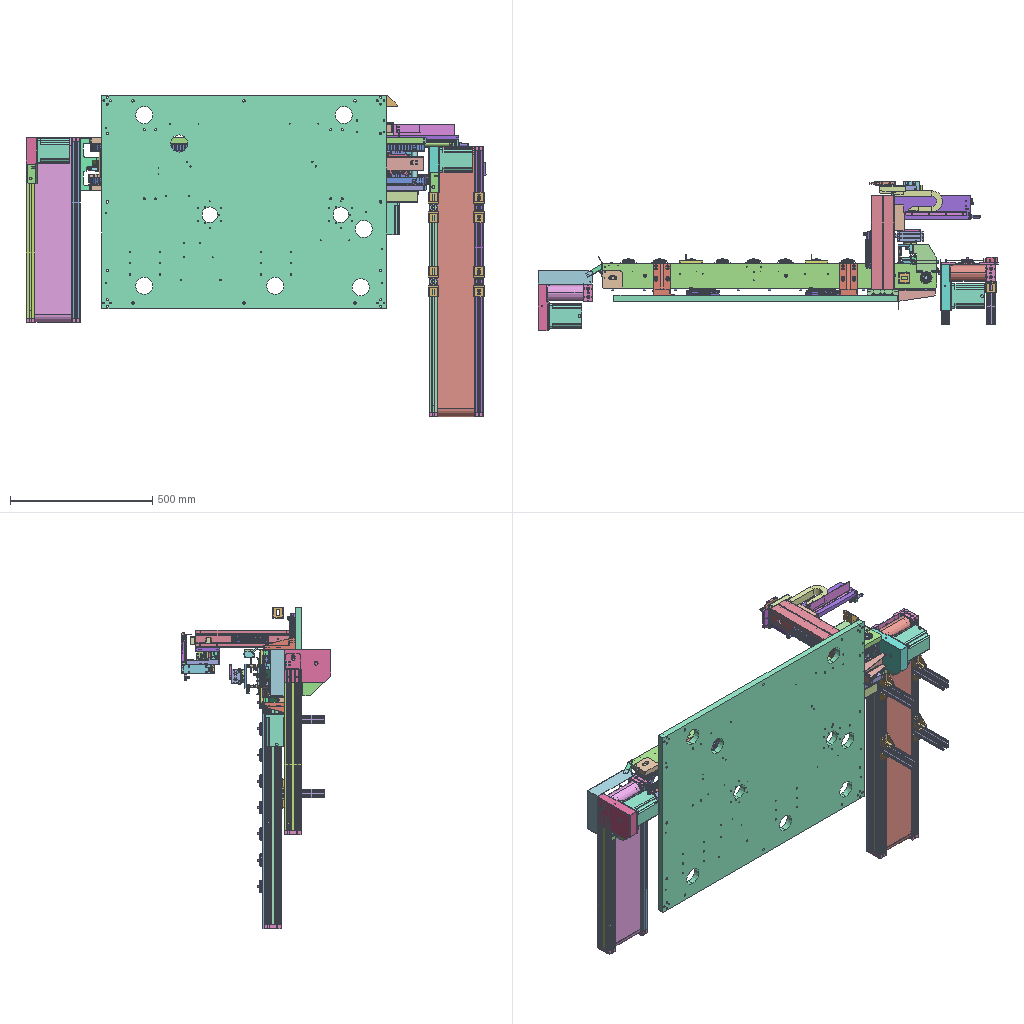Assembly | STEP file | 114 different items | 249 placed | box 1615 x 525 x 1130 mm
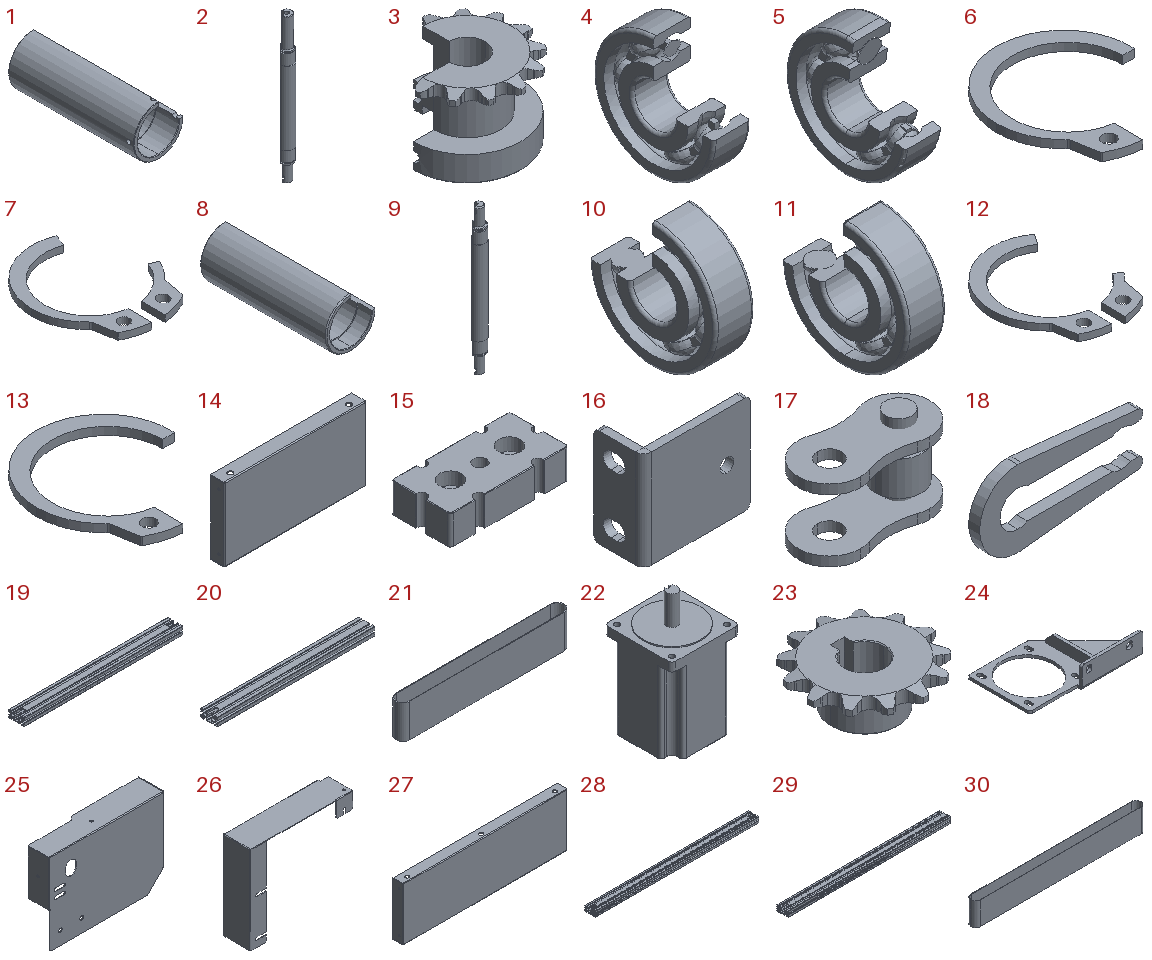Parts list (item | name | quantity | parent item | size | volume):
1 | - | x2 | - | 50 x 126 x 50 mm | 63059 mm3
2 | drive shaft | x2 | - | 16 x 16 x 176 mm | 21338 mm3
3 | driven sprocket | x2 | - | 44.21 x 43.904 x 30.003 mm | 14979 mm3
4 | Bearing 6302 | x2 | - | 13 x 42 x 42 mm | 7777 mm3
5 | Bearing 6302 | x2 | - | 13 x 41.82 x 42 mm | 7834 mm3
6 | Shaft retaining ring type A 15 | x2 | - | 16.8 x 19.352 x 1 mm | 66.829 mm3
7 | Shaft retaining ring type A 15 | x2 | - | 16.068 x 19.352 x 1 mm | 68.849 mm3
8 | - | x2 | - | 50 x 126 x 50 mm | 63952 mm3
9 | driven shaft | x2 | - | 16 x 15.999 x 170 mm | 21183 mm3
10 | Bearing 6302 | x2 | - | 13 x 42 x 42 mm | 7890 mm3
11 | Bearing 6302 | x2 | - | 13 x 41.997 x 42 mm | 7881 mm3
12 | Shaft retaining ring type A 15 | x2 | - | 15.123 x 19.352 x 1 mm | 70.172 mm3
13 | Shaft retaining ring type A 15 | x2 | - | 16.8 x 19.352 x 1 mm | 66.829 mm3
14 | - | x2 | - | 250 x 25 x 130 mm | 74457 mm3
15 | B2200 end cap_zinc alloy | x6 | - | 60 x 30 x 15 mm | 23538 mm3
16 | drive wheel fixing plate | x2 | - | 54.501 x 25.501 x 50 mm | 14216 mm3
17 | Industrial chain 06B-1-160 links | x2 | - | 18.125 x 8.6 x 12.32 mm | 522.22 mm3
18 | Chain link 3 (06B) | x2 | - | 15 x 1 x 7 mm | 49.292 mm3
19 | belt line support ET profile 620 | x1 | - | 620 x 60 x 30 mm | 399085 mm3
20 | belt line support ET profile 565 | x1 | - | 565 x 60 x 30 mm | 364592 mm3
21 | Light green PVC conveyor belt 1346x129x2mm thick_antistatic | x1 | - | 648.5 x 54 x 129 mm | 348910 mm3
22 | Stepper motor 34HS4801D14PJ5 | x3 | in HJ conveyor line assembly | 86 x 89 x 152.5 mm | 773985 mm3
23 | Drive sprocket 06B-13 teeth_bore φ14 | x2 | - | 44.21 x 43.904 x 16.003 mm | 7455 mm3
24 | - | x2 | - | 160 x 100 x 32 mm | 46086 mm3
25 | sprocket guard | x1 | - | 163 x 35.5 x 116 mm | 28902 mm3
26 | - | x1 | - | 190 x 50 x 163 mm | 24970 mm3
27 | belt support plate | x2 | - | 400 x 25 x 130 mm | 113936 mm3
28 | belt line support ET profile 920 | x1 | - | 920 x 60 x 30 mm | 594868 mm3
29 | - | x1 | - | 865 x 60 x 30 mm | 559855 mm3
30 | Light green PVC conveyor belt 1946x129x2mm thick_antistatic | x1 | - | 948.5 x 54 x 129 mm | 503710 mm3
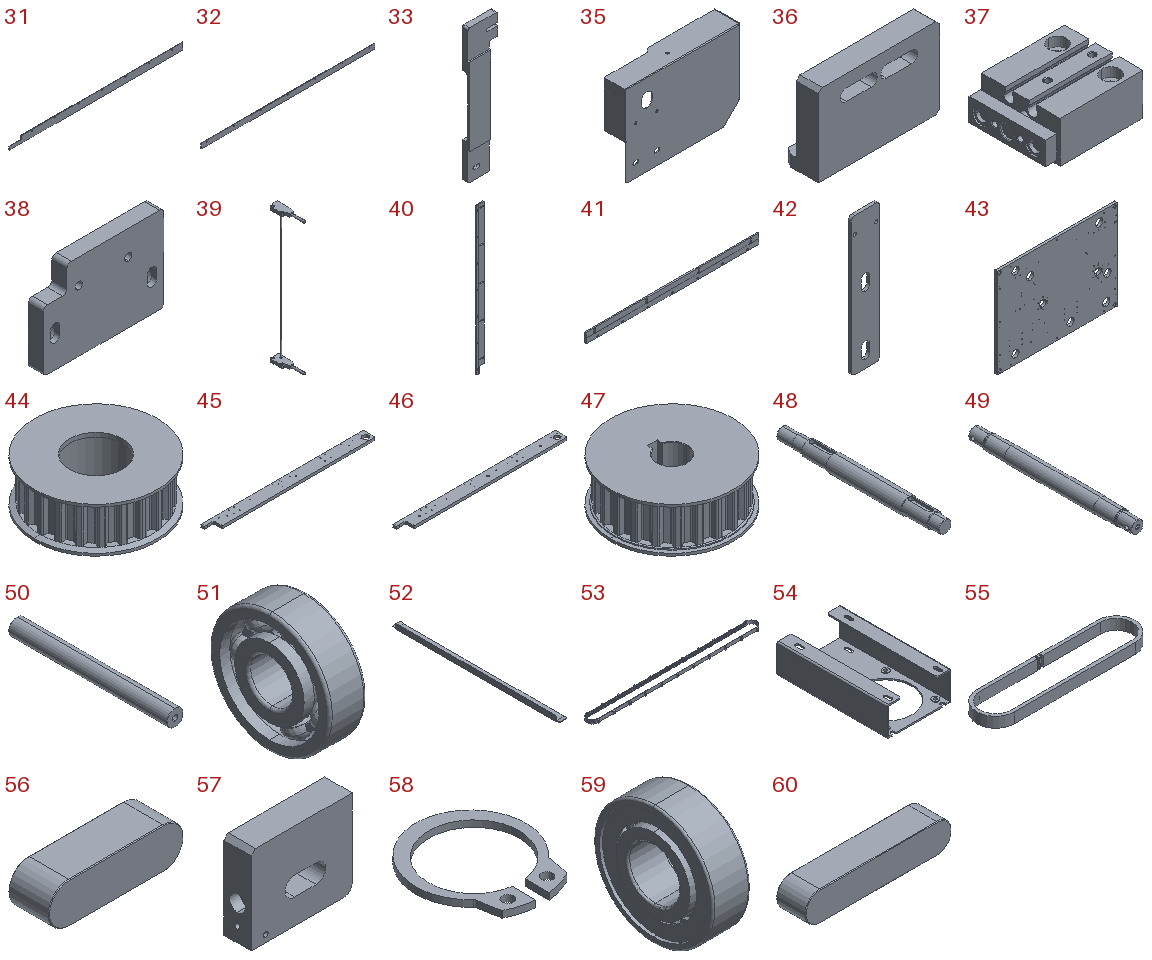31 | BZJ-BZMM-JDKTBDYY Product限位Plate一 | x1 | - | 890 x 2 x 35 mm | 59822 mm3
32 | BZJ-BZMM-JDKTBDYY Product限位Plate二 | x1 | - | 895 x 2 x 26 mm | 46280 mm3
33 | - | x1 | - | 42 x 10 x 190 mm | 34788 mm3
34 | product | x21 | in gripper rotary assembly | - | -
35 | motor fixing plate | x1 | - | 163 x 35.5 x 116 mm | 28996 mm3
36 | secondary positioning block | x1 | - | 33 x 9.454 x 22 mm | 4103 mm3
37 | Three-axis cylinder TCM10x10S | x1 | - | - | -
38 | - | x1 | - | 56 x 7 x 40 mm | 13740 mm3
39 | Through-beam ultra-thin photoelectric switch EX-11A_150 | x1 | - | 10 x 35.5 x 157 mm | 1436 mm3
40 | BZJ-BZMM-JDKTBDYY Product限位Plate四 | x1 | - | 44 x 6 x 895 mm | 219689 mm3
41 | BZJ-BZMM-JDKTBDYY Product限位Plate三 | x1 | - | 830 x 6 x 48 mm | 225450 mm3
42 | through-beam photoelectric fixing plate | x2 | - | 14.5 x 1.5 x 70 mm | 1416 mm3
43 | - | x1 | - | 1000 x 22 x 750 mm | 15887768 mm3
44 | Timing pulley 22-T10-φ35-27 | x2 | in HJ conveyor line assembly | 74 x 74 x 27 mm | 67542 mm3
45 | - | x1 | in HJ conveyor line assembly | 1175 x 85 x 19 mm | 1776717 mm3
46 | - | x1 | in HJ conveyor line assembly | 1175 x 85 x 19 mm | 1780086 mm3
47 | Timing pulley 22-T10-φ18-27 | x2 | in HJ conveyor line assembly | 74 x 74 x 27 mm | 85142 mm3
48 | - | x1 | in HJ conveyor line assembly | 20 x 198 x 20 mm | 50387 mm3
49 | - | x1 | in HJ conveyor line assembly | 16 x 176 x 16 mm | 31579 mm3
50 | - | x3 | in HJ conveyor line assembly | 15 x 147 x 15 mm | 25052 mm3
51 | Bearing 6302 | x2 | in HJ conveyor line assembly | 13 x 42 x 42 mm | 10445 mm3
52 | T10 timing belt support plate | x4 | in HJ conveyor line assembly | 25.5 x 510.959 x 15 mm | 29071 mm3
53 | Timing belt with stop block 2420-T10-21mm wide | x2 | in HJ conveyor line assembly | 1172 x 86.18 x 21.9 mm | 158627 mm3
54 | 86 motor mounting flange | x1 | in HJ conveyor line assembly | 90 x 155 x 41 mm | 53412 mm3
55 | Timing belt 270-3M-8mm wide_28-28 teeth H93 | x1 | in HJ conveyor line assembly | 122.34 x 29.34 x 8 mm | 5374 mm3
56 | Type A key 6x6 20L | x2 | in HJ conveyor line assembly | 20 x 6 x 6 mm | 673.18 mm3
57 | adjustment limit plate | x2 | in HJ conveyor line assembly | 70 x 19 x 60 mm | 70894 mm3
58 | Shaft retaining ring type A 15 | x2 | in HJ conveyor line assembly | 16.8 x 19.352 x 1 mm | 89.212 mm3
59 | Bearing 6202-2Z | x4 | in HJ conveyor line assembly | 11 x 35 x 35 mm | 5288 mm3
60 | Plain key type A 5x5x25 | x1 | in HJ conveyor line assembly | 25 x 5 x 5 mm | 597.62 mm3
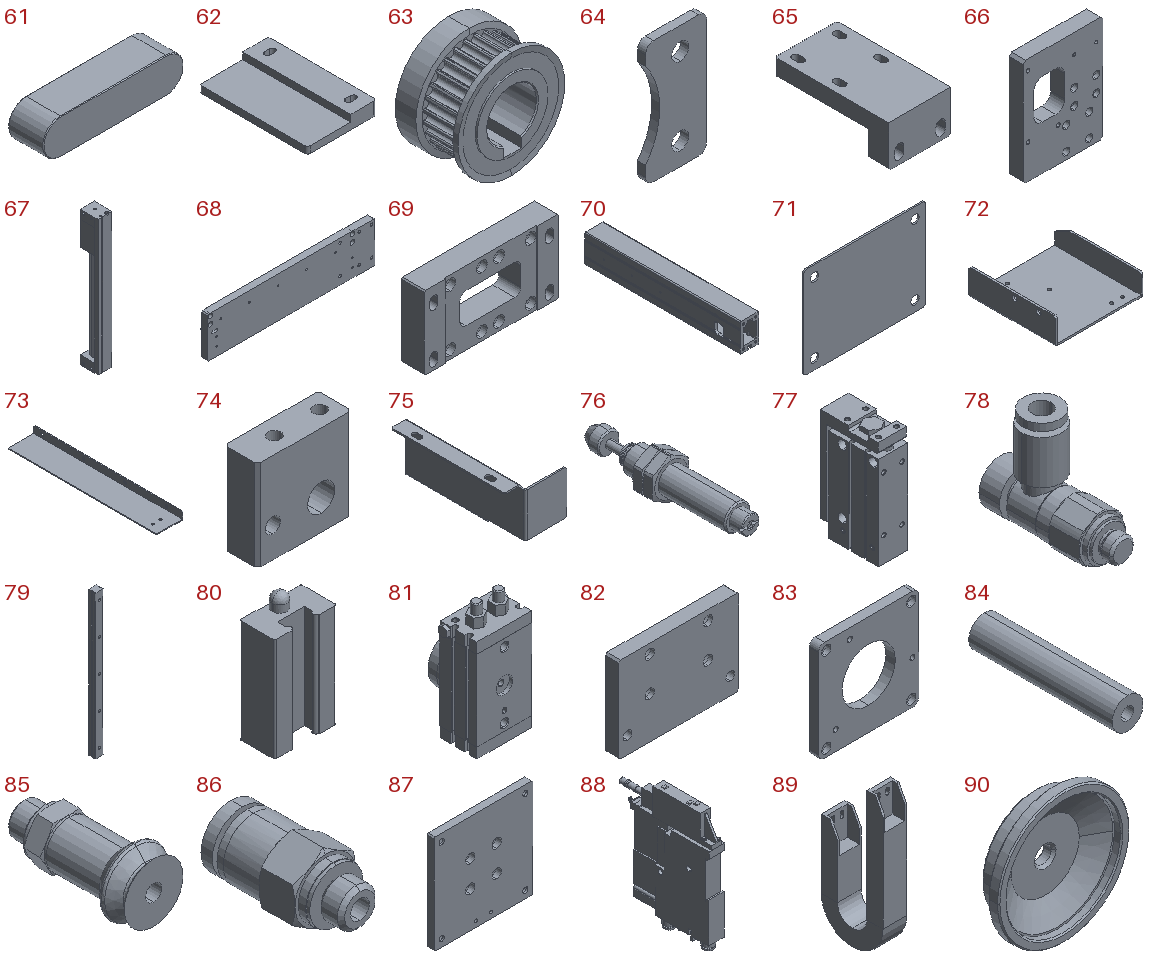61 | Plain key (type B) 5x5x20 | x1 | in HJ conveyor line assembly | 20 x 5 x 5 mm | 472.72 mm3
62 | - | x4 | in HJ conveyor line assembly | 51 x 80 x 10 mm | 27378 mm3
63 | Timing pulley 28-3M-φ14-19-J | x2 | in HJ conveyor line assembly | 30 x 19 x 30 mm | 7318 mm3
64 | - | x2 | in HJ conveyor line assembly | 15 x 2 x 30 mm | 737.571 mm3
65 | - | x4 | - | 60 x 110 x 40 mm | 130636 mm3
66 | slide fixing plate | x1 | in gripper rotary assembly | 90 x 24 x 120 mm | 159761 mm3
67 | Magnetically coupled rodless cylinder CY3R15-200 | x1 | in gripper rotary assembly | 32 x 40 x 294 mm | 185652 mm3
68 | - | x1 | in gripper rotary assembly | 350 x 14 x 85 mm | 395442 mm3
69 | - | x1 | in gripper rotary assembly | 110 x 19 x 60 mm | 87261 mm3
70 | - | x2 | in gripper rotary assembly | 40 x 330 x 60 mm | 402728 mm3
71 | 4060 profile end cover plate | x1 | in gripper rotary assembly | 80 x 1 x 60 mm | 4702 mm3
72 | drag chain fixing plate | x1 | in gripper rotary assembly | 91 x 90 x 27 mm | 24044 mm3
73 | drag chain support plate | x1 | in gripper rotary assembly | 38 x 215 x 11 mm | 12174 mm3
74 | - | x2 | in gripper rotary assembly | 31 x 11 x 30 mm | 8762 mm3
75 | - | x1 | in gripper rotary assembly | 42 x 90 x 36.2 mm | 8185 mm3
76 | Hydraulic shock absorber ACA1007-2 | x2 | in gripper rotary assembly | 14 x 62 x 15.686 mm | 4586 mm3
77 | Pneumatic slide MXH20-50Z_with magnet_no sensor | x1 | in gripper rotary assembly | 32 x 64.5 x 118 mm | 192171 mm3
78 | Speed control valve AS1201F-M5-04A | x4 | in gripper rotary assembly | 9.373 x 25.4 x 22 mm | 1869 mm3
79 | Guide rail SSR15XW1SSC1+270LY | x1 | in 79 | 15 x 12.5 x 270 mm | 46741 mm3
80 | Slider 15_THK_SSR15XW | x1 | in 79 | 34 x 19.5 x 65 mm | 30926 mm3
81 | Swing table MSQB10A | x1 | in gripper rotary assembly | 55.4 x 47 x 109.81 mm | 167301 mm3
82 | swing table fixing plate | x1 | in gripper rotary assembly | 70 x 8 x 50 mm | 25661 mm3
83 | - | x1 | - | 85 x 8 x 85 mm | 43514 mm3
84 | connecting column | x4 | - | 8 x 37 x 8 mm | 1657 mm3
85 | Vacuum suction cup ZPT08BS-A5_longitudinal vacuum outlet type_no buffer_bellows type | x3 | - | 10 x 20 x 10 mm | 691.38 mm3
86 | Quick-change joint KQ2H04-M5A | x3 | - | 8 x 17 x 9.238 mm | 543.469 mm3
87 | - | x1 | - | 85 x 6 x 85 mm | 41251 mm3
88 | Vacuum generator ZK2A10K5KW-06 | x1 | in gripper rotary assembly | - | -
89 | JFLO drag chain 15.20B, bend radius R28 | x1 | in gripper rotary assembly | 28.5 x 74.5 x 172.25 mm | 143432 mm3
90 | - | x1 | in gripper rotary assembly | 55 x 12.5 x 55 mm | 12038 mm3
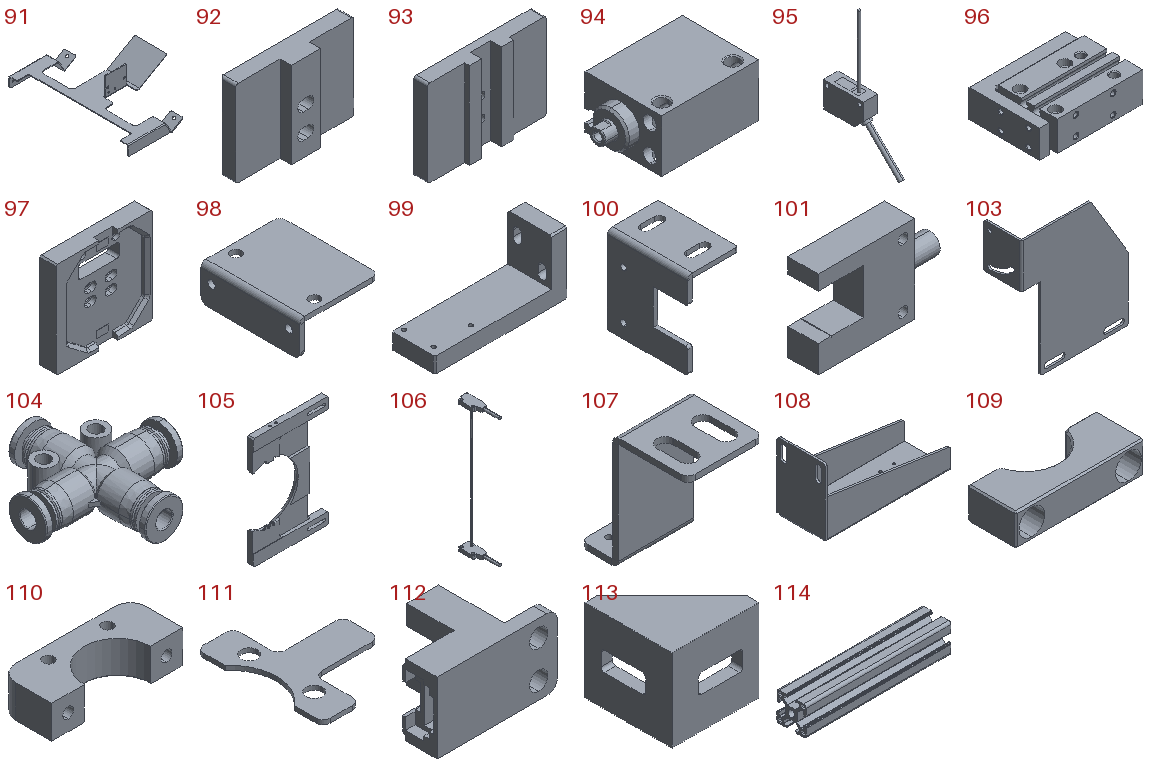91 | unloading flow plate | x1 | - | 128.223 x 185 x 46.263 mm | 15132 mm3
92 | product positioning block | x2 | - | 48 x 12.5 x 35 mm | 13200 mm3
93 | product positioning block B | x30 | - | 48 x 10 x 35 mm | 11917 mm3
94 | Compact free-mount cylinder MU6x6S | x1 | - | 30 x 19 x 13 mm | 4914 mm3
95 | Compact photoelectric sensor CX-441 | x4 | in lift assembly | 11.2 x 58.715 x 100.215 mm | 7246 mm3
96 | Compact pneumatic slide MXH6-15Z | x2 | in lift assembly | 54.5 x 39 x 16 mm | 25990 mm3
97 | lift positioning block | x2 | in lift assembly | 70 x 12 x 70 mm | 41545 mm3
98 | lift photoelectric fixing plate | x2 | in lift assembly | 25.5 x 32 x 11.5 mm | 1639 mm3
99 | cylinder fixing plate 2 | x2 | in lift assembly | 85 x 28 x 40 mm | 31178 mm3
100 | photoelectric mounting plate | x1 | - | 22 x 35 x 38 mm | 3386 mm3
101 | Photoelectric sensor SU15-N | x1 | - | 42 x 11.5 x 29 mm | 7150 mm3
102 | I/O junction box 23N8S1 | x3 | - | - | -
103 | photoelectric fixing plate 2 | x1 | - | 85 x 30 x 100 mm | 11300 mm3
104 | Tube fitting PZ4 | x1 | - | 34 x 34 x 9.5 mm | 2906 mm3
105 | material release guide plate | x1 | - | 125 x 10 x 185 mm | 96002 mm3
106 | Through-beam ultra-thin photoelectric switch EX-11A_120 | x1 | - | 10 x 35.5 x 127 mm | 1412 mm3
107 | - | x2 | - | 20 x 28.5 x 30 mm | 1546 mm3
108 | - | x1 | - | 130 x 50 x 70 mm | 33645 mm3
109 | photoelectric switch fixing block 1 | x1 | - | 40 x 15 x 10 mm | 3490 mm3
110 | photoelectric switch fixing plate 2 | x1 | - | 40 x 16 x 10 mm | 4339 mm3
111 | - | x1 | - | 28 x 35 x 1.2 mm | 521.608 mm3
112 | Photoelectric sensor PM-Y65 | x1 | - | 22.7 x 14.9 x 13.4 mm | 1660 mm3
113 | Die-cast aluminium connector, 40 series, 40mm face, standard type | x9 | - | 38 x 38 x 36 mm | 14409 mm3
114 | MK-8-3030-L-00 profile 3030 standard type 150mm | x4 | - | 150 x 30 x 30 mm | 48990 mm3
Placements (level | parent | child | x y z in mm | rotation matrix by rows):
1 | subassembly 2 | subassembly 3 | -12.345 572.465 974.383 | 1 0 9e-06 0 -1 0 9e-06 0 -1
2 | subassembly 3 | subassembly 4 | -203.579 -184.273 737.895 | 0 1 0 -1 0 0 0 0 1
3 | subassembly 4 | subassembly 5 | -56.737 26.612 373.0 | 1 0 0 0 1 0 0 0 1
3 | subassembly 4 | drive shaft | -56.737 23.612 373.0 | 0 1 0 0 0 -1 -1 0 -0
3 | subassembly 4 | driven sprocket | -56.737 -54.242 373.0 | 0 1 0 0 0 -1 -1 0 0
3 | subassembly 4 | Bearing 6302 | -56.737 -19.888 373.0 | 0 -1 0 1 0 0 0 0 1
3 | subassembly 4 | Bearing 6302 | -56.737 82.112 373.0 | 0 -0.9914 -0.1307 1 0 0 0 -0.1307 0.9914
3 | subassembly 4 | Shaft retaining ring type A 15 | -56.737 -26.888 372.5 | 1 0 0 0 0 1 0 -1 0
3 | subassembly 4 | Shaft retaining ring type A 15 | -56.27 89.112 372.822 | 0.357 0.9341 0 0 0 1 0.9341 -0.357 0
2 | subassembly 3 | subassembly 6 | -196.548 -168.949 1359.395 | 0 -1 0 1 0 0 0 0 1
3 | subassembly 6 | subassembly 7 | 41.413 -19.581 346.0 | 1 0 0 0 1 0 0 0 1
3 | subassembly 6 | driven shaft | 41.413 -19.581 346.0 | 0.01582 0.9999 0 0 0 -1 -0.9999 0.01582 0
3 | subassembly 6 | Bearing 6302 | 41.413 35.919 346.0 | 0 1 0 -1 0 0 0 0 1
3 | subassembly 6 | Bearing 6302 | 41.413 -75.081 346.0 | 0 0.9998 -0.01821 -1 0 0 0 0.01821 0.9998
3 | subassembly 6 | Shaft retaining ring type A 15 | 41.828 -82.081 345.72 | 0.5593 0.829 0 0 0 1 0.829 -0.5593 -0
3 | subassembly 6 | Shaft retaining ring type A 15 | 41.413 42.919 345.5 | 1 0 0 0 0 1 0 -1 0
2 | subassembly 3 | subassembly 8 | -176.967 -151.036 1541.203 | 0 0 1 0 1 0 -1 0 -0
2 | subassembly 3 | subassembly 8 | -176.967 -151.036 1291.203 | 0 0 1 0 1 0 -1 0 -0
2 | subassembly 3 | B2200 end cap_zinc alloy | -96.967 -127.535 1090.896 | 0 1 0 1 0 0 0 0 -1
2 | subassembly 3 | B2200 end cap_zinc alloy | -256.967 -127.535 1725.896 | 0 -1 0 1 0 0 0 0 1
2 | subassembly 3 | B2200 end cap_zinc alloy | -96.967 -127.535 1725.896 | 0 -1 0 1 0 0 0 0 1
2 | subassembly 3 | drive wheel fixing plate | -267.967 -127.535 1098.895 | 0 1 0 0 0 -1 -1 0 -0
2 | subassembly 3 | Industrial chain 06B-1-160 links | -267.89 -45.475 1101.33 | 0 0 -1 0.9905 -0.1375 0 -0.1375 -0.9905 0
2 | subassembly 3 | Chain link 3 (06B) | -262.761 -50.192 1101.984 | 0 -1 0 -0.9905 0 -0.1375 0.1375 0 -0.9905
2 | subassembly 3 | belt line support ET profile 620 | -96.967 -142.536 1408.396 | 0 0 -1 0 -1 0 -1 0 0
2 | subassembly 3 | belt line support ET profile 565 | -256.967 -112.535 1435.896 | 0 0 1 0 1 0 -1 0 -0
2 | subassembly 3 | Light green PVC conveyor belt 1346x129x2mm thick_antistatic | -176.967 -127.535 1408.145 | 0 0 1 0 1 0 -1 0 -0
2 | subassembly 3 | Stepper motor 34HS4801D14PJ5 | -119.967 -46.035 1131.396 | 0 0 -1 1 0 0 0 -1 -0
2 | subassembly 3 | Drive sprocket 06B-13 teeth_bore φ14 | -257.821 -46.035 1131.396 | 0 0 -1 -0.9914 0.1312 0 0.1312 0.9914 -0
2 | subassembly 3 | subassembly 9 | -237.967 -42.535 1131.396 | 0 0 -1 0 1 0 1 0 0
2 | subassembly 3 | sprocket guard | -271.967 -156.536 1084.396 | 0 1 0 1 0 0 0 0 -1
2 | subassembly 3 | subassembly 10 | -271.967 -182.536 1083.396 | 1 0 0 0 -1 0 0 0 -1
1 | subassembly 2 | subassembly 11 | 1122.454 698.033 793.393 | 0 -1 9e-06 -1 0 0 0 -9e-06 -1
2 | subassembly 11 | subassembly 4 | -128.705 -75.924 587.895 | -1 0 0 0 -1 0 0 0 1
3 | subassembly 4 | subassembly 5 | -56.737 26.612 373.0 | 1 0 0 0 1 0 0 0 1
3 | subassembly 4 | drive shaft | -56.737 23.612 373.0 | 0 1 0 0 0 -1 -1 0 -0
3 | subassembly 4 | driven sprocket | -56.737 -54.242 373.0 | 0 1 0 0 0 -1 -1 0 0
3 | subassembly 4 | Bearing 6302 | -56.737 -19.888 373.0 | 0 -1 0 1 0 0 0 0 1
3 | subassembly 4 | Bearing 6302 | -56.737 82.112 373.0 | 0 -0.9914 -0.1307 1 0 0 0 -0.1307 0.9914
3 | subassembly 4 | Shaft retaining ring type A 15 | -56.737 -26.888 372.5 | 1 0 0 0 0 1 0 -1 0
3 | subassembly 4 | Shaft retaining ring type A 15 | -56.27 89.112 372.822 | 0.357 0.9341 0 0 0 1 0.9341 -0.357 0
2 | subassembly 11 | subassembly 6 | -113.38 -82.954 1509.395 | 1 0 0 0 1 0 0 0 1
3 | subassembly 6 | subassembly 7 | 41.413 -19.581 346.0 | 1 0 0 0 1 0 0 0 1
3 | subassembly 6 | driven shaft | 41.413 -19.581 346.0 | 0.01582 0.9999 0 0 0 -1 -0.9999 0.01582 0
3 | subassembly 6 | Bearing 6302 | 41.413 35.919 346.0 | 0 1 0 -1 0 0 0 0 1
3 | subassembly 6 | Bearing 6302 | 41.413 -75.081 346.0 | 0 0.9998 -0.01821 -1 0 0 0 0.01821 0.9998
3 | subassembly 6 | Shaft retaining ring type A 15 | 41.828 -82.081 345.72 | 0.5593 0.829 0 0 0 1 0.829 -0.5593 -0
3 | subassembly 6 | Shaft retaining ring type A 15 | 41.413 42.919 345.5 | 1 0 0 0 0 1 0 -1 0
2 | subassembly 11 | belt support plate | -95.467 -102.535 1603.396 | 0 1 0 0 0 -1 -1 0 0
2 | subassembly 11 | belt support plate | -95.467 -102.535 1203.396 | 0 1 0 0 0 -1 -1 0 0
2 | subassembly 11 | B2200 end cap_zinc alloy | -71.967 -182.536 940.896 | -1 0 0 0 1 0 0 0 -1
2 | subassembly 11 | B2200 end cap_zinc alloy | -71.967 -22.535 1875.896 | 1 0 0 0 1 0 0 0 1
2 | subassembly 11 | B2200 end cap_zinc alloy | -71.967 -182.536 1875.896 | 1 0 0 0 1 0 0 0 1
2 | subassembly 11 | drive wheel fixing plate | -71.967 -11.536 948.895 | 0 0 -1 0 -1 0 -1 0 0
2 | subassembly 11 | Industrial chain 06B-1-160 links | 19.686 -26.615 960.264 | 0.7485 0.6631 0 6e-06 -6e-06 1 0.6631 -0.7485 -9e-06
2 | subassembly 11 | Chain link 3 (06B) | 16.121 -31.744 957.106 | -0.7485 0 0.6631 -6e-06 1 -6e-06 -0.6631 -9e-06 -0.7485
2 | subassembly 11 | belt line support ET profile 920 | -86.967 -182.536 1408.396 | 0 -1 0 0 0 1 -1 0 0
2 | subassembly 11 | subassembly 12 | -56.967 -22.535 1435.896 | 0 1 0 0 0 -1 -1 0 0
2 | subassembly 11 | Light green PVC conveyor belt 1946x129x2mm thick_antistatic | -71.967 -102.535 1408.145 | 0 1 0 0 0 -1 -1 0 0
2 | subassembly 11 | BZJ-BZMM-JDKTBDYY Product限位Plate一 | -100.467 -144.536 1438.396 | 0 -1 0 0 0 -1 1 0 0
2 | subassembly 11 | BZJ-BZMM-JDKTBDYY Product限位Plate二 | -102.467 -55.035 1435.896 | 0 1 0 0 0 1 1 0 0
2 | subassembly 11 | subassembly 13 | -101.967 -102.535 948.396 | 0 -1 0 0 0 -1 1 0 -0
2 | subassembly 11 | product | -91.767 -183.843 927.176 | -1 0 0 0 1 -0.001005 0 -0.001005 -1
2 | subassembly 11 | motor fixing plate | -100.967 -7.535 934.396 | 1 0 0 0 -1 0 0 0 -1
2 | subassembly 11 | subassembly 9 | 13.033 -41.535 981.396 | 0 1 0 0 0 1 1 0 0
2 | subassembly 11 | Stepper motor 34HS4801D14PJ5 | 9.533 -159.536 981.396 | 1 0 0 0 0 1 0 -1 -0
2 | subassembly 11 | Drive sprocket 06B-13 teeth_bore φ14 | 9.533 -21.682 981.396 | -0.9892 0.1467 0 0 0 1 0.1467 0.9892 0
2 | subassembly 11 | secondary positioning block | -110.467 -159.536 1007.596 | 0 0 -1 0 1 0 1 0 -0
2 | subassembly 11 | Three-axis cylinder TCM10x10S | -116.467 -168.536 1007.596 | 0 0 -1 -1 0 0 0 1 -0
2 | subassembly 11 | subassembly 14 | -101.967 -187.536 1007.596 | 0 -1 0 0 0 -1 1 0 -0
2 | subassembly 11 | Through-beam ultra-thin photoelectric switch EX-11A_150 | -118.967 -181.036 988.604 | -1 0 0 0 0 1 0 1 0
2 | subassembly 11 | BZJ-BZMM-JDKTBDYY Product限位Plate四 | -101.967 -29.535 1435.896 | 0 -1 0 1 0 0 0 0 1
2 | subassembly 11 | BZJ-BZMM-JDKTBDYY Product限位Plate三 | -101.967 -173.536 1468.396 | 0 -1 0 0 0 -1 1 0 0
2 | subassembly 11 | through-beam photoelectric fixing plate | -83.967 -197.536 995.854 | 0 0 -1 0 1 0 1 0 0
2 | subassembly 11 | through-beam photoelectric fixing plate | -83.967 -5.035 995.854 | 0 0 -1 0 1 0 1 0 0
1 | subassembly 2 | subassembly 15 | 480 692.0 -335.008 | 1 0 -9e-06 0 1 0 9e-06 0 1
2 | subassembly 15 | subassembly 16 | -0.0 -0.0 -0.0 | 1 0 0 0 1 0 0 0 1
2 | subassembly 15 | HJ conveyor line assembly | -178.498 50.792 136.934 | 1 0 0 0 1 0 0 0 1
3 | HJ conveyor line assembly | Timing pulley 22-T10-φ35-27 | -324.002 10.208 -63.434 | -0.3841 0.9233 0 -0.9233 -0.3841 0 0 0 1
3 | HJ conveyor line assembly | Timing pulley 22-T10-φ35-27 | -324.002 10.208 54.566 | 0.06596 -0.9978 0 -0.9978 -0.06596 0 0 0 -1
3 | HJ conveyor line assembly | subassembly 17 | 225.998 16.708 -87.434 | 1 0 0 0 1 0 0 0 1
3 | HJ conveyor line assembly | subassembly 18 | 225.998 16.708 78.566 | 1 0 0 0 1 0 0 0 1
3 | HJ conveyor line assembly | Timing pulley 22-T10-φ18-27 | 775.997 10.208 -63.434 | 0.043 -0.9991 0 0.9991 0.043 0 0 0 1
3 | HJ conveyor line assembly | Timing pulley 22-T10-φ18-27 | 775.997 10.208 54.566 | 0.043 -0.9991 0 0.9991 0.043 0 0 0 1
3 | HJ conveyor line assembly | subassembly 19 | 775.997 10.208 -4.434 | 0.043 0 -0.9991 0.9991 0 0.043 0 -1 0
3 | HJ conveyor line assembly | subassembly 20 | -324.002 10.208 -4.434 | -1 0 0 0 0 1 0 1 0
3 | HJ conveyor line assembly | subassembly 21 | -211.502 16.708 -4.434 | 0.9491 0 0.3149 0.3149 0 -0.9491 0 1 0
3 | HJ conveyor line assembly | subassembly 21 | 283.498 16.708 -4.434 | 0.5837 0 -0.812 -0.812 0 -0.5837 0 1 -0
3 | HJ conveyor line assembly | subassembly 21 | 663.497 16.708 -4.434 | 1 0 0 0 0 -1 0 1 0
3 | HJ conveyor line assembly | Bearing 6302 | 775.997 10.208 78.566 | 0 0.8011 0.5985 0 0.5985 -0.8011 -1 0 0
3 | HJ conveyor line assembly | Bearing 6302 | 775.997 10.208 -87.434 | 0 0.8065 0.5913 0 0.5913 -0.8065 -1 0 0
3 | HJ conveyor line assembly | T10 timing belt support plate | -30.003 41.708 -77.934 | 0 -1 0 0 0 -1 1 0 0
3 | HJ conveyor line assembly | T10 timing belt support plate | 481.998 41.708 -77.934 | 0 -1 0 0 0 -1 1 0 0
3 | HJ conveyor line assembly | Timing belt with stop block 2420-T10-21mm wide | -324.002 10.208 -62.734 | 1 0 0 0 1 0 0 0 1
3 | HJ conveyor line assembly | Timing belt with stop block 2420-T10-21mm wide | -324.002 10.208 53.866 | 1 0 0 0 -1 0 0 0 -1
3 | HJ conveyor line assembly | T10 timing belt support plate | -30.003 41.708 69.066 | 0 1 0 0 0 -1 -1 0 0
3 | HJ conveyor line assembly | T10 timing belt support plate | 481.998 41.708 69.066 | 0 1 0 0 0 -1 -1 0 0
3 | HJ conveyor line assembly | Stepper motor 34HS4801D14PJ5 | 680.497 14.208 -251.934 | 0 -1 0 1 0 0 0 0 1
3 | HJ conveyor line assembly | 86 motor mounting flange | 710.997 14.208 -137.934 | 0 1 0 -1 0 0 0 0 1
3 | HJ conveyor line assembly | Timing belt 270-3M-8mm wide_28-28 teeth H93 | 683.084 14.208 -115.198 | 0.9991 0.04301 0 -0.04301 0.9991 0 0 0 1
3 | HJ conveyor line assembly | Type A key 6x6 20L | 767.805 10.56 51.066 | 0 -0.9991 0.043 0 0.043 0.9991 -1 0 -0
3 | HJ conveyor line assembly | Type A key 6x6 20L | 767.805 10.56 -59.934 | 0 -0.9991 0.043 0 0.043 0.9991 -1 0 -0
3 | HJ conveyor line assembly | adjustment limit plate | -326.502 4.208 -87.434 | 1 0 0 0 0 -1 0 1 0
3 | HJ conveyor line assembly | adjustment limit plate | -326.502 4.208 78.566 | 1 0 0 0 0 -1 0 1 0
3 | HJ conveyor line assembly | Shaft retaining ring type A 15 | -324.002 10.708 -74.934 | 1 0 0 0 1 0 0 0 1
3 | HJ conveyor line assembly | Shaft retaining ring type A 15 | -324.002 10.708 66.066 | 1 0 0 0 1 0 0 0 1
3 | HJ conveyor line assembly | Bearing 6202-2Z | -324.002 10.208 -57.934 | 0 -0.437 0.8995 0 0.8995 0.437 -1 0 0
3 | HJ conveyor line assembly | Bearing 6202-2Z | -324.002 10.208 -68.934 | 0 0 1 0 1 0 -1 0 0
3 | HJ conveyor line assembly | Bearing 6202-2Z | -324.002 10.208 49.066 | 0 0.02822 0.9996 0 0.9996 -0.02822 -1 0 0
3 | HJ conveyor line assembly | Bearing 6202-2Z | -324.002 10.208 60.066 | 0 0.7582 0.6521 0 0.6521 -0.7582 -1 0 0
3 | HJ conveyor line assembly | Plain key type A 5x5x25 | 673.997 14.208 -111.934 | 0 -1 0 0 0 1 -1 0 0
3 | HJ conveyor line assembly | Plain key (type B) 5x5x20 | 782.491 9.928 -102.934 | 0 -0.9991 0.043 0 0.043 0.9991 -1 0 -0
3 | HJ conveyor line assembly | subassembly 22 | 430.998 59.208 69.066 | 0 -1 0 0 0 -1 1 0 0
3 | HJ conveyor line assembly | subassembly 22 | 350.998 59.208 -77.934 | 0 1 0 0 0 -1 -1 0 0
3 | HJ conveyor line assembly | subassembly 22 | -9.002 59.208 69.066 | 0 -1 0 0 0 -1 1 0 0
3 | HJ conveyor line assembly | subassembly 22 | -89.002 59.208 -77.934 | 0 1 0 0 0 -1 -1 0 0
3 | HJ conveyor line assembly | Timing pulley 28-3M-φ14-19-J | 775.997 10.208 -106.434 | -0.4924 0 -0.8704 -0.8704 0 0.4924 0 1 0
3 | HJ conveyor line assembly | Timing pulley 28-3M-φ14-19-J | 680.497 14.208 -105.934 | 0.9991 0 0.04278 -0.04278 0 0.9991 0 -1 0
3 | HJ conveyor line assembly | subassembly 23 | 797.497 10.208 -95.267 | 1 0 0 0 0 1 0 -1 0
3 | HJ conveyor line assembly | subassembly 23 | 754.497 10.208 -97.267 | -1 0 0 0 0 1 0 1 -0
2 | subassembly 15 | subassembly 24 | -330.0 55.0 240.0 | -1 0 0 0 1 0 0 0 -1
2 | subassembly 15 | subassembly 24 | 325.0 55.0 240.0 | -1 0 0 0 1 0 0 0 -1
2 | subassembly 15 | subassembly 24 | -330.0 55.0 25.0 | 1 0 0 0 1 0 0 0 1
2 | subassembly 15 | subassembly 24 | 325.0 55.0 25.0 | 1 0 0 0 1 0 0 0 1
2 | subassembly 15 | gripper rotary assembly | 846.194 181.79 160.616 | -1 0 0 0 1 0 0 0 -1
3 | gripper rotary assembly | slide fixing plate | 326.694 143.21 -19.884 | 1 0 0 0 0 1 0 -1 0
3 | gripper rotary assembly | Magnetically coupled rodless cylinder CY3R15-200 | 379.694 140.21 -42.884 | 0 0 1 0 -1 0 1 0 0
3 | gripper rotary assembly | subassembly 25 | 266.194 125.71 -65.884 | 1 0 0 0 0 -1 0 1 -0
3 | gripper rotary assembly | subassembly 26 | 401.194 -172.29 -102.884 | 1 0 0 0 1 0 0 0 1
3 | gripper rotary assembly | subassembly 27 | 421.194 2.21 -102.884 | 1 0 0 0 -1 0 0 0 -1
3 | gripper rotary assembly | subassembly 27 | 381.194 2.21 -102.884 | 1 0 0 0 -1 0 0 0 -1
3 | gripper rotary assembly | 4060 profile end cover plate | 401.194 167.21 -102.884 | 1 0 0 0 1 0 0 0 1
3 | gripper rotary assembly | drag chain fixing plate | 366.694 201.21 -116.884 | 0 1 0 0 0 -1 -1 0 -0
3 | gripper rotary assembly | drag chain support plate | 213.194 110.21 -110.884 | 0 -1 0 0 0 -1 1 0 -0
3 | gripper rotary assembly | subassembly 28 | 96.694 98.71 -44.884 | 0 -1 0 -1 0 0 0 0 -1
3 | gripper rotary assembly | subassembly 28 | 393.694 98.71 -44.884 | 0 -1 0 -1 0 0 0 0 -1
3 | gripper rotary assembly | subassembly 29 | 361.194 88.71 -112.684 | 0 0 1 0 -1 0 1 0 0
3 | gripper rotary assembly | Hydraulic shock absorber ACA1007-2 | 430.194 93.21 -39.884 | 0 -1 0 0.9922 0 0.1244 -0.1244 0 0.9922
3 | gripper rotary assembly | Hydraulic shock absorber ACA1007-2 | 57.194 93.21 -39.884 | 0 1 0 -1 0 0 0 0 1
3 | gripper rotary assembly | Pneumatic slide MXH20-50Z_with magnet_no sensor | 304.194 115.71 4.116 | 0 -1 0 0 0 -1 1 0 -0
3 | gripper rotary assembly | Speed control valve AS1201F-M5-04A | 288.194 203.21 20.116 | 0.6488 0 0.7609 0.7609 0 -0.6488 0 1 0
3 | gripper rotary assembly | Speed control valve AS1201F-M5-04A | 320.194 203.21 20.116 | 0.6488 0 0.7609 0.7609 0 -0.6488 0 1 0
3 | gripper rotary assembly | Speed control valve AS1201F-M5-04A | 398.694 140.21 -42.884 | 0 1 0 0.8937 0 -0.4486 -0.4486 0 -0.8937
3 | gripper rotary assembly | Speed control valve AS1201F-M5-04A | 104.694 140.21 -42.884 | 0 -1 0 0.4991 0 0.8666 -0.8666 0 0.4991
3 | gripper rotary assembly | Guide rail SSR15XW1SSC1+270LY | 238.194 104.21 -47.384 | 0 0 1 1 0 0 0 1 0
4 | Guide rail SSR15XW1SSC1+270LY | Guide rail SSR15XW1SSC1+270LY | -0.0 0.0 -0.0 | 1 0 0 0 1 0 0 0 1
4 | Guide rail SSR15XW1SSC1+270LY | Slider 15_THK_SSR15XW | -0.0 0.0 -58.5 | 1 0 0 0 1 0 0 0 1
3 | gripper rotary assembly | Swing table MSQB10A | 304.194 42.21 28.616 | 0 0 1 0 -1 0 1 0 0
3 | gripper rotary assembly | swing table fixing plate | 304.194 50.21 13.616 | 1 0 0 0 -1 0 0 0 -1
3 | gripper rotary assembly | subassembly 30 | 192.235 -6.363 53.852 | 1 0 0 0 1 0 0 0 1
4 | subassembly 30 | subassembly 31 | 111.96 -49.428 -25.236 | 1 0 0 0 1 0 0 0 1
4 | subassembly 30 | connecting column | 75.96 -41.428 10.764 | 1 0 0 0 1 0 0 0 1
4 | subassembly 30 | connecting column | 147.959 -41.428 10.764 | 1 0 0 0 1 0 0 0 1
4 | subassembly 30 | connecting column | 147.959 -41.428 -61.236 | 1 0 0 0 1 0 0 0 1
4 | subassembly 30 | connecting column | 75.96 -41.428 -61.236 | 1 0 0 0 1 0 0 0 1
4 | subassembly 30 | Vacuum suction cup ZPT08BS-A5_longitudinal vacuum outlet type_no buffer_bellows type | 83.96 -65.927 -51.236 | 0.4402 0 -0.8979 0 1 0 0.8979 0 0.4402
4 | subassembly 30 | Vacuum suction cup ZPT08BS-A5_longitudinal vacuum outlet type_no buffer_bellows type | 148.959 -65.927 -31.236 | 0.9884 0 -0.1516 0 1 0 0.1516 0 0.9884
4 | subassembly 30 | Vacuum suction cup ZPT08BS-A5_longitudinal vacuum outlet type_no buffer_bellows type | 95.96 -65.927 8.764 | 0.9745 0 -0.2245 0 1 0 0.2245 0 0.9745
4 | subassembly 30 | Quick-change joint KQ2H04-M5A | 95.96 -41.428 8.764 | 1 0 0 0 1 0 0 0 1
4 | subassembly 30 | Quick-change joint KQ2H04-M5A | 148.959 -41.428 -31.236 | 1 0 0 0 1 0 0 0 1
4 | subassembly 30 | Quick-change joint KQ2H04-M5A | 83.96 -41.428 -51.236 | 1 0 0 0 1 0 0 0 1
4 | subassembly 30 | subassembly 32 | 111.96 -4.428 -25.236 | -1 0 0 0 1 0 0 0 -1
3 | gripper rotary assembly | Vacuum generator ZK2A10K5KW-06 | 354.794 210.71 -98.184 | 0 1 0 1 0 0 0 0 -1
3 | gripper rotary assembly | JFLO drag chain 15.20B, bend radius R28 | 363.694 174.96 -95.884 | 0 0 1 0 -1 0 1 0 0
3 | gripper rotary assembly | product | 373.478 -81.29 -55.035 | 0 0.001004 1 1 0 0 0 1 -0.001004
3 | gripper rotary assembly | subassembly 33 | 304.194 -60.29 28.616 | 0.9836 0 -0.1801 0 1 0 0.1801 0 0.9836
2 | subassembly 15 | unloading flow plate | -565.115 76.7 132.5 | 0.866 0 0.5 0.5 0 -0.866 0 1 0
2 | subassembly 15 | product | 473.216 96.09 216.151 | 0 -0.001005 -1 1 0 0 0 -1 0.001005
2 | subassembly 15 | product | 363.216 96.09 216.151 | 0 -0.001005 -1 1 0 0 0 -1 0.001005
2 | subassembly 15 | product | 253.216 96.09 216.151 | 0 -0.001005 -1 1 0 0 0 -1 0.001005
2 | subassembly 15 | product | 143.216 96.09 216.151 | 0 -0.001005 -1 1 0 0 0 -1 0.001005
2 | subassembly 15 | product | 33.216 96.09 216.151 | 0 -0.001005 -1 1 0 0 0 -1 0.001005
2 | subassembly 15 | product | -76.784 96.09 216.151 | 0 -0.001005 -1 1 0 0 0 -1 0.001005
2 | subassembly 15 | product | -186.784 96.09 216.151 | 0 -0.001005 -1 1 0 0 0 -1 0.001005
2 | subassembly 15 | product | -296.784 96.09 216.151 | 0 -0.001005 -1 1 0 0 0 -1 0.001005
2 | subassembly 15 | product | -406.784 96.09 216.151 | 0 -0.001005 -1 1 0 0 0 -1 0.001005
2 | subassembly 15 | product | -516.784 96.09 216.151 | 0 -0.001005 -1 1 0 0 0 -1 0.001005
2 | subassembly 15 | product positioning block | -521.388 98.452 79.325 | 0.8745 -0.485 0 0.485 0.8745 0 0 0 1
2 | subassembly 15 | product positioning block B | 542.5 101.59 79.325 | 1 0 0 0 1 0 0 0 1
2 | subassembly 15 | product positioning block B | 542.5 101.59 185.675 | -1 0 0 0 1 0 0 0 -1
2 | subassembly 15 | product positioning block B | 432.5 101.59 185.675 | -1 0 0 0 1 0 0 0 -1
2 | subassembly 15 | product positioning block B | 322.5 101.59 185.675 | -1 0 0 0 1 0 0 0 -1
2 | subassembly 15 | product positioning block B | 212.5 101.59 185.675 | -1 0 0 0 1 0 0 0 -1
2 | subassembly 15 | product positioning block B | 102.5 101.59 185.675 | -1 0 0 0 1 0 0 0 -1
2 | subassembly 15 | product positioning block B | -7.5 101.59 185.675 | -1 0 0 0 1 0 0 0 -1
2 | subassembly 15 | product positioning block B | -117.5 101.59 185.675 | -1 0 0 0 1 0 0 0 -1
2 | subassembly 15 | product positioning block B | -227.5 101.59 185.675 | -1 0 0 0 1 0 0 0 -1
2 | subassembly 15 | product positioning block B | -337.5 101.59 185.675 | -1 0 0 0 1 0 0 0 -1
2 | subassembly 15 | product positioning block B | -447.5 101.59 185.675 | -1 0 0 0 1 0 0 0 -1
2 | subassembly 15 | product positioning block B | 432.5 101.59 79.325 | 1 0 0 0 1 0 0 0 1
2 | subassembly 15 | product positioning block B | 322.5 101.59 79.325 | 1 0 0 0 1 0 0 0 1
2 | subassembly 15 | product positioning block B | 212.5 101.59 79.325 | 1 0 0 0 1 0 0 0 1
2 | subassembly 15 | product positioning block B | 102.5 101.59 79.325 | 1 0 0 0 1 0 0 0 1
2 | subassembly 15 | product positioning block B | -7.5 101.59 79.325 | 1 0 0 0 1 0 0 0 1
2 | subassembly 15 | product positioning block B | -117.5 101.59 79.325 | 1 0 0 0 1 0 0 0 1
2 | subassembly 15 | product positioning block B | -227.5 101.59 79.325 | 1 0 0 0 1 0 0 0 1
2 | subassembly 15 | product positioning block B | -337.5 101.59 79.325 | 1 0 0 0 1 0 0 0 1
2 | subassembly 15 | product positioning block B | -447.5 101.59 79.325 | 1 0 0 0 1 0 0 0 1
2 | subassembly 15 | Compact free-mount cylinder MU6x6S | -524.809 91.888 138.0 | 0.5 0 -0.866 -0.866 0 -0.5 0 1 0
2 | subassembly 15 | Compact photoelectric sensor CX-441 | -526.074 89.079 115.9 | 0 -0.866 -0.5 0 -0.5 0.866 -1 0 0
2 | subassembly 15 | lift assembly | 420.226 163.431 -5.601 | 0 0 -1 -1 0 0 0 1 0
3 | lift assembly | Compact pneumatic slide MXH6-15Z | 79.431 136.813 207.726 | 1 0 0 0 1 0 0 0 1
3 | lift assembly | lift positioning block | 58.931 138.163 207.726 | 0 1 0 -1 0 0 0 0 1
3 | lift assembly | Compact photoelectric sensor CX-441 | 75.931 144.663 225.626 | 0 0 -1 0 -1 0 -1 0 0
3 | lift assembly | lift photoelectric fixing plate | 72.431 154.163 242.726 | 1 0 0 0 -1 0 0 0 -1
3 | lift assembly | cylinder fixing plate 2 | 153.431 152.163 159.726 | 1 0 0 0 -1 0 0 0 -1
2 | subassembly 15 | lift assembly | -19.774 163.431 -5.601 | 0 0 -1 -1 0 0 0 1 0
3 | lift assembly | Compact pneumatic slide MXH6-15Z | 79.431 136.813 207.726 | 1 0 0 0 1 0 0 0 1
3 | lift assembly | lift positioning block | 58.931 138.163 207.726 | 0 1 0 -1 0 0 0 0 1
3 | lift assembly | Compact photoelectric sensor CX-441 | 75.931 144.663 225.626 | 0 0 -1 0 -1 0 -1 0 0
3 | lift assembly | lift photoelectric fixing plate | 72.431 154.163 242.726 | 1 0 0 0 -1 0 0 0 -1
3 | lift assembly | cylinder fixing plate 2 | 153.431 152.163 159.726 | 1 0 0 0 -1 0 0 0 -1
2 | subassembly 15 | photoelectric mounting plate | -307.0 2.0 108.0 | 1 0 0 0 0 -1 0 1 -0
2 | subassembly 15 | Photoelectric sensor SU15-N | -314.0 21.4 106.3 | 0 -1 0 0 0 -1 1 0 0
2 | subassembly 15 | product positioning block | -337.5 17.91 79.325 | -1 0 0 0 -1 0 0 0 1
2 | subassembly 15 | I/O junction box 23N8S1 | -178.77 0.85 291.892 | -0.6592 -0.752 0 0 0 1 -0.752 0.6592 0
2 | subassembly 15 | Compact photoelectric sensor CX-441 | 544.4 155.5 198.5 | -1 0 0 0 1 0 0 0 -1
2 | subassembly 15 | photoelectric fixing plate 2 | 600.0 129.5 225.0 | 1 0 0 0 0 1 0 -1 0
2 | subassembly 15 | I/O junction box 23N8S1 | 241.73 0.85 291.892 | -0.6592 -0.752 0 0 0 1 -0.752 0.6592 0
2 | subassembly 15 | I/O junction box 23N8S1 | 404.15 149.55 263.5 | 0 0 -1 0 1 0 1 0 -0
2 | subassembly 15 | Tube fitting PZ4 | 541.823 166.5 87.827 | 0.9996 0.02692 0 0 0 -1 -0.02692 0.9996 -0
2 | subassembly 15 | material release guide plate | 577.5 110.0 132.5 | 1 0 0 0 1 0 0 0 1
2 | subassembly 15 | product positioning block B | 597.5 101.59 78.325 | 1 0 -1e-06 0 1 0 1e-06 0 1
2 | subassembly 15 | product positioning block B | 601.038 101.436 78.325 | 0.9962 0.08716 -1e-06 -0.08716 0.9962 0 1e-06 0 1
2 | subassembly 15 | product positioning block B | 604.548 100.973 78.325 | 0.9848 0.1736 -1e-06 -0.1736 0.9848 0 1e-06 0 1
2 | subassembly 15 | product positioning block B | 608.005 100.207 78.325 | 0.9659 0.2588 -1e-06 -0.2588 0.9659 0 1e-06 0 1
2 | subassembly 15 | product positioning block B | 611.383 99.142 78.325 | 0.9397 0.342 -1e-06 -0.342 0.9397 0 1e-06 0 1
2 | subassembly 15 | product positioning block B | 614.654 97.787 78.325 | 0.9063 0.4226 -1e-06 -0.4226 0.9063 1e-06 1e-06 0 1
2 | subassembly 15 | product positioning block B | 617.795 96.152 78.325 | 0.866 0.5 -1e-06 -0.5 0.866 1e-06 1e-06 0 1
2 | subassembly 15 | product positioning block B | 620.782 94.249 78.325 | 0.8192 0.5736 -1e-06 -0.5736 0.8192 1e-06 1e-06 0 1
2 | subassembly 15 | product positioning block B | 623.591 92.094 78.325 | 0.766 0.6428 -1e-06 -0.6428 0.766 1e-06 1e-06 0 1
2 | subassembly 15 | product positioning block B | 626.202 89.701 78.325 | 0.7071 0.7071 -1e-06 -0.7071 0.7071 1e-06 1e-06 0 1
2 | subassembly 15 | Through-beam ultra-thin photoelectric switch EX-11A_120 | 559.5 124.0 196.0 | 0 -1 0 -1 0 0 0 0 -1
2 | subassembly 15 | subassembly 34 | 552.25 130.25 67.0 | -1 0 0 0 1 0 0 0 -1
2 | subassembly 15 | subassembly 34 | 552.25 130.25 198.0 | 1 0 0 0 1 0 0 0 1
2 | subassembly 15 | subassembly 35 | 565.0 16.718 133.6 | 1 0 0 0 0 -1 0 1 0
2 | subassembly 15 | photoelectric switch fixing block 1 | 597.994 70.487 127.5 | -0.9986 -0.05196 0 0.05196 -0.9986 0 0 0 1
2 | subassembly 15 | photoelectric switch fixing plate 2 | 597.5 61.0 127.5 | -0.9986 -0.05196 0 0.05196 -0.9986 0 0 0 1
2 | subassembly 15 | subassembly 36 | 579.712 55.917 138.7 | -0.05196 0.9986 0 -0.9986 -0.05196 0 0 0 1
2 | subassembly 15 | Photoelectric sensor PM-Y65 | 597.0 31.618 141.1 | -1 0 0 0 1 0 0 0 -1
1 | subassembly 2 | product | 1306.205 789.8 -133.204 | 0 -1 0.000997 1 0 0 0 0.000997 1
1 | subassembly 2 | product | 1306.205 789.8 -225.504 | 0 -1 0.000997 1 0 0 0 0.000997 1
1 | subassembly 2 | product | 1306.206 789.8 -317.804 | 0 -1 0.000997 1 0 0 0 0.000997 1
1 | subassembly 2 | product | 1306.207 789.8 -410.104 | 0 -1 0.000997 1 0 0 0 0.000997 1
1 | subassembly 2 | product | 1306.208 789.8 -502.404 | 0 -1 0.000997 1 0 0 0 0.000997 1
1 | subassembly 2 | product | 1306.209 789.8 -594.704 | 0 -1 0.000997 1 0 0 0 0.000997 1
1 | subassembly 2 | product | 1306.209 789.8 -687.004 | 0 -1 0.000997 1 0 0 0 0.000997 1
1 | subassembly 2 | product | 1306.21 789.8 -779.304 | 0 -1 0.000997 1 0 0 0 0.000997 1
1 | subassembly 2 | product | 1306.211 789.8 -871.604 | 0 -1 0.000997 1 0 0 0 0.000997 1
1 | subassembly 2 | Die-cast aluminium connector, 40 series, 40mm face, standard type | 980.0 752.0 0.0001 | 0 1 0 0 0 1 1 0 0
1 | subassembly 2 | MK-8-3030-L-00 profile 3030 standard type 150mm | 1304.999 590 -355.002 | 0 -1 -9e-06 1 0 0 0 -9e-06 1
1 | subassembly 2 | MK-8-3030-L-00 profile 3030 standard type 150mm | 1144.999 590 -355.002 | 0 -1 -9e-06 1 0 0 0 -9e-06 1
1 | subassembly 2 | Die-cast aluminium connector, 40 series, 40mm face, standard type | 1144.999 740.0 -340.002 | 0 -9e-06 -1 -1 0 0 0 1 -9e-06
1 | subassembly 2 | Die-cast aluminium connector, 40 series, 40mm face, standard type | 1304.999 740.0 -340.001 | 0 -9e-06 -1 -1 0 0 0 1 -9e-06
1 | subassembly 2 | Die-cast aluminium connector, 40 series, 40mm face, standard type | 1305.002 740.0 -600.001 | 0 -9e-06 -1 -1 0 0 0 1 -9e-06
1 | subassembly 2 | Die-cast aluminium connector, 40 series, 40mm face, standard type | 1145.002 740.0 -600.002 | 0 -9e-06 -1 -1 0 0 0 1 -9e-06
1 | subassembly 2 | MK-8-3030-L-00 profile 3030 standard type 150mm | 1145.002 590 -615.002 | 0 -1 -9e-06 1 0 0 0 -9e-06 1
1 | subassembly 2 | MK-8-3030-L-00 profile 3030 standard type 150mm | 1305.002 590 -615.002 | 0 -1 -9e-06 1 0 0 0 -9e-06 1
1 | subassembly 2 | Die-cast aluminium connector, 40 series, 40mm face, standard type | 1305 740.0 -370.003 | 0 9e-06 1 -1 0 0 0 -1 9e-06
1 | subassembly 2 | Die-cast aluminium connector, 40 series, 40mm face, standard type | 1145 740.0 -370.005 | 0 9e-06 1 -1 0 0 0 -1 9e-06
1 | subassembly 2 | Die-cast aluminium connector, 40 series, 40mm face, standard type | 1145.002 740.0 -630.005 | 0 9e-06 1 -1 0 0 0 -1 9e-06
1 | subassembly 2 | Die-cast aluminium connector, 40 series, 40mm face, standard type | 1305.002 740.0 -630.003 | 0 9e-06 1 -1 0 0 0 -1 9e-06